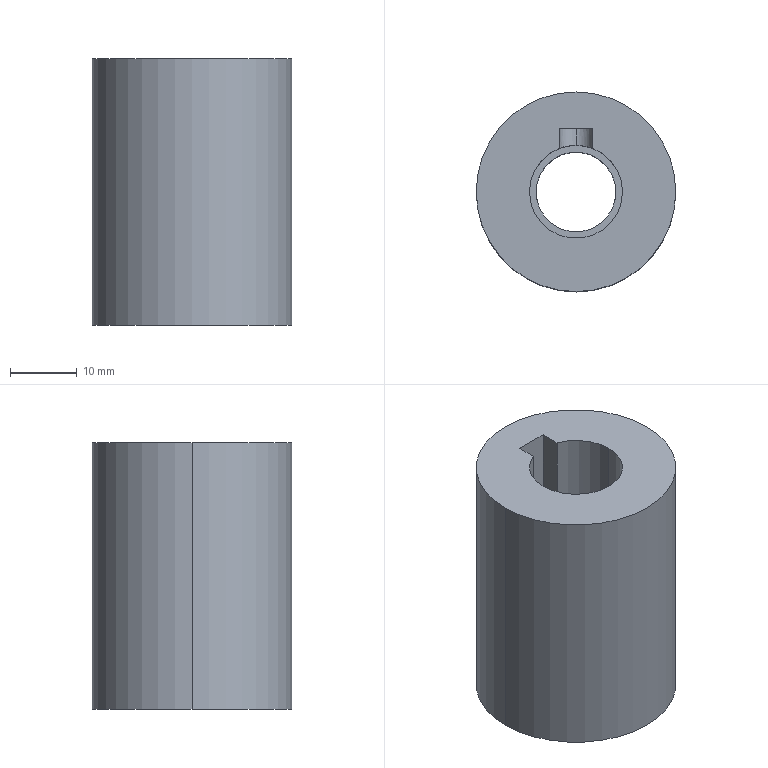Part | 1 solid | 19 faces | box 30 x 30 x 40 mm | volume 22641 mm3 | cylinder 10 | plane 9 | commonest cylinder face diameters 4 x2 5 x2 12 x2 14 x2 30 x2
STEP:
#1=CARTESIAN_POINT('',(-7.,0.,20.));
#2=VERTEX_POINT('',#1);
#3=CARTESIAN_POINT('',(7.,0.,20.));
#4=VERTEX_POINT('',#3);
#5=CARTESIAN_POINT('',(0.,0.,20.));
#6=DIRECTION('',(0.,0.,1.));
#7=DIRECTION('',(1.,0.,0.));
#8=AXIS2_PLACEMENT_3D('',#5,#6,#7);
#9=CIRCLE('',#8,7.);
#10=EDGE_CURVE('',#2,#4,#9,.T.);
#11=ORIENTED_EDGE('',*,*,#10,.T.);
#12=CARTESIAN_POINT('',(7.,0.,0.));
#13=VERTEX_POINT('',#12);
#14=CARTESIAN_POINT('',(7.,0.,20.));
#15=DIRECTION('',(0.,0.,-1.));
#16=VECTOR('',#15,1000.);
#17=LINE('',#14,#16);
#18=EDGE_CURVE('',#4,#13,#17,.T.);
#19=ORIENTED_EDGE('',*,*,#18,.T.);
#20=CARTESIAN_POINT('',(-7.,0.,0.));
#21=VERTEX_POINT('',#20);
#22=CARTESIAN_POINT('',(0.,0.,0.));
#23=DIRECTION('',(0.,0.,1.));
#24=DIRECTION('',(1.,0.,0.));
#25=AXIS2_PLACEMENT_3D('',#22,#23,#24);
#26=CIRCLE('',#25,7.);
#27=EDGE_CURVE('',#21,#13,#26,.T.);
#28=ORIENTED_EDGE('',*,*,#27,.F.);
#29=CARTESIAN_POINT('',(-7.,0.,20.));
#30=DIRECTION('',(0.,0.,-1.));
#31=VECTOR('',#30,1000.);
#32=LINE('',#29,#31);
#33=EDGE_CURVE('',#2,#21,#32,.T.);
#34=ORIENTED_EDGE('',*,*,#33,.F.);
#35=EDGE_LOOP('',(#11,#19,#28,#34));
#36=FACE_OUTER_BOUND('',#35,.T.);
#37=CARTESIAN_POINT('',(0.,0.,20.));
#38=DIRECTION('',(0.,0.,-1.));
#39=DIRECTION('',(-1.,0.,0.));
#40=AXIS2_PLACEMENT_3D('',#37,#38,#39);
#41=CYLINDRICAL_SURFACE('',#40,7.);
#42=ADVANCED_FACE('',(#36),#41,.F.);
#43=CARTESIAN_POINT('',(15.,0.,20.));
#44=VERTEX_POINT('',#43);
#45=CARTESIAN_POINT('',(-15.,0.,20.));
#46=VERTEX_POINT('',#45);
#47=CARTESIAN_POINT('',(0.,0.,20.));
#48=DIRECTION('',(0.,0.,1.));
#49=DIRECTION('',(1.,0.,0.));
#50=AXIS2_PLACEMENT_3D('',#47,#48,#49);
#51=CIRCLE('',#50,15.);
#52=EDGE_CURVE('',#44,#46,#51,.T.);
#53=ORIENTED_EDGE('',*,*,#52,.F.);
#54=CARTESIAN_POINT('',(15.,0.,-20.));
#55=VERTEX_POINT('',#54);
#56=CARTESIAN_POINT('',(15.,0.,20.));
#57=DIRECTION('',(0.,0.,-1.));
#58=VECTOR('',#57,1000.);
#59=LINE('',#56,#58);
#60=EDGE_CURVE('',#44,#55,#59,.T.);
#61=ORIENTED_EDGE('',*,*,#60,.T.);
#62=CARTESIAN_POINT('',(-15.,0.,-20.));
#63=VERTEX_POINT('',#62);
#64=CARTESIAN_POINT('',(0.,0.,-20.));
#65=DIRECTION('',(0.,0.,-1.));
#66=DIRECTION('',(-1.,0.,0.));
#67=AXIS2_PLACEMENT_3D('',#64,#65,#66);
#68=CIRCLE('',#67,15.);
#69=EDGE_CURVE('',#63,#55,#68,.T.);
#70=ORIENTED_EDGE('',*,*,#69,.F.);
#71=CARTESIAN_POINT('',(-15.,0.,20.));
#72=DIRECTION('',(0.,0.,-1.));
#73=VECTOR('',#72,1000.);
#74=LINE('',#71,#73);
#75=EDGE_CURVE('',#46,#63,#74,.T.);
#76=ORIENTED_EDGE('',*,*,#75,.F.);
#77=EDGE_LOOP('',(#53,#61,#70,#76));
#78=FACE_OUTER_BOUND('',#77,.T.);
#79=CARTESIAN_POINT('',(0.,0.,20.));
#80=DIRECTION('',(0.,0.,-1.));
#81=DIRECTION('',(-1.,0.,0.));
#82=AXIS2_PLACEMENT_3D('',#79,#80,#81);
#83=CYLINDRICAL_SURFACE('',#82,15.);
#84=ADVANCED_FACE('',(#78),#83,.T.);
#85=CARTESIAN_POINT('',(-2.,-5.657,-20.));
#86=VERTEX_POINT('',#85);
#87=CARTESIAN_POINT('',(-6.,0.,-20.));
#88=VERTEX_POINT('',#87);
#89=CARTESIAN_POINT('',(0.,0.,-20.));
#90=DIRECTION('',(0.,0.,-1.));
#91=DIRECTION('',(-1.,0.,0.));
#92=AXIS2_PLACEMENT_3D('',#89,#90,#91);
#93=CIRCLE('',#92,6.);
#94=EDGE_CURVE('',#86,#88,#93,.T.);
#95=ORIENTED_EDGE('',*,*,#94,.T.);
#96=CARTESIAN_POINT('',(-6.,0.,0.));
#97=VERTEX_POINT('',#96);
#98=CARTESIAN_POINT('',(-6.,0.,-20.));
#99=DIRECTION('',(0.,0.,1.));
#100=VECTOR('',#99,1000.);
#101=LINE('',#98,#100);
#102=EDGE_CURVE('',#88,#97,#101,.T.);
#103=ORIENTED_EDGE('',*,*,#102,.T.);
#104=CARTESIAN_POINT('',(6.,0.,0.));
#105=VERTEX_POINT('',#104);
#106=CARTESIAN_POINT('',(0.,0.,0.));
#107=DIRECTION('',(0.,0.,-1.));
#108=DIRECTION('',(-1.,0.,0.));
#109=AXIS2_PLACEMENT_3D('',#106,#107,#108);
#110=CIRCLE('',#109,6.);
#111=EDGE_CURVE('',#105,#97,#110,.T.);
#112=ORIENTED_EDGE('',*,*,#111,.F.);
#113=CARTESIAN_POINT('',(6.,0.,-20.));
#114=VERTEX_POINT('',#113);
#115=CARTESIAN_POINT('',(6.,0.,-20.));
#116=DIRECTION('',(0.,0.,1.));
#117=VECTOR('',#116,1000.);
#118=LINE('',#115,#117);
#119=EDGE_CURVE('',#114,#105,#118,.T.);
#120=ORIENTED_EDGE('',*,*,#119,.F.);
#121=CARTESIAN_POINT('',(2.,-5.657,-20.));
#122=VERTEX_POINT('',#121);
#123=CARTESIAN_POINT('',(0.,0.,-20.));
#124=DIRECTION('',(0.,0.,-1.));
#125=DIRECTION('',(-1.,0.,0.));
#126=AXIS2_PLACEMENT_3D('',#123,#124,#125);
#127=CIRCLE('',#126,6.);
#128=EDGE_CURVE('',#114,#122,#127,.T.);
#129=ORIENTED_EDGE('',*,*,#128,.T.);
#130=CARTESIAN_POINT('',(2.,-5.657,-8.));
#131=VERTEX_POINT('',#130);
#132=CARTESIAN_POINT('',(2.,-5.657,-6.));
#133=DIRECTION('',(0.,0.,-1.));
#134=VECTOR('',#133,1000.);
#135=LINE('',#132,#134);
#136=EDGE_CURVE('',#131,#122,#135,.T.);
#137=ORIENTED_EDGE('',*,*,#136,.F.);
#138=CARTESIAN_POINT('',(0.,-6.,-6.));
#139=VERTEX_POINT('',#138);
#140=CARTESIAN_POINT('',(2.,-5.657,-8.));
#141=CARTESIAN_POINT('',(2.,-5.657,-7.867));
#142=CARTESIAN_POINT('',(1.987,-5.662,-7.736));
#143=CARTESIAN_POINT('',(1.936,-5.679,-7.479));
#144=CARTESIAN_POINT('',(1.897,-5.693,-7.352));
#145=CARTESIAN_POINT('',(1.796,-5.725,-7.11));
#146=CARTESIAN_POINT('',(1.735,-5.744,-6.996));
#147=CARTESIAN_POINT('',(1.59,-5.786,-6.779));
#148=CARTESIAN_POINT('',(1.506,-5.809,-6.678));
#149=CARTESIAN_POINT('',(1.232,-5.875,-6.403));
#150=CARTESIAN_POINT('',(1.01,-5.919,-6.255));
#151=CARTESIAN_POINT('',(0.6502,-5.966,-6.104));
#152=CARTESIAN_POINT('',(0.5235,-5.979,-6.065));
#153=CARTESIAN_POINT('',(0.2644,-5.996,-6.013));
#154=CARTESIAN_POINT('',(0.1331,-6.,-6.));
#155=CARTESIAN_POINT('',(0.,-6.,-6.));
#156=B_SPLINE_CURVE_WITH_KNOTS('',3,(#140,#141,#142,#143,#144,#145,#146,#147,#148,#149,#150,#151,#152,#153,#154,#155),.UNSPECIFIED.,.F.,.F.,(4,2,2,2,2,2,2,4),(0.,0.0003934,0.0007868,0.00118,0.001574,0.00236,0.002754,0.003147),.UNSPECIFIED.);
#157=EDGE_CURVE('',#131,#139,#156,.T.);
#158=ORIENTED_EDGE('',*,*,#157,.T.);
#159=CARTESIAN_POINT('',(-2.,-5.657,-8.));
#160=VERTEX_POINT('',#159);
#161=CARTESIAN_POINT('',(0.,-6.,-6.));
#162=CARTESIAN_POINT('',(-0.1331,-6.,-6.));
#163=CARTESIAN_POINT('',(-0.2638,-5.996,-6.013));
#164=CARTESIAN_POINT('',(-0.5206,-5.979,-6.065));
#165=CARTESIAN_POINT('',(-0.6481,-5.966,-6.103));
#166=CARTESIAN_POINT('',(-0.8898,-5.935,-6.204));
#167=CARTESIAN_POINT('',(-1.004,-5.916,-6.266));
#168=CARTESIAN_POINT('',(-1.221,-5.876,-6.411));
#169=CARTESIAN_POINT('',(-1.323,-5.853,-6.494));
#170=CARTESIAN_POINT('',(-1.597,-5.787,-6.769));
#171=CARTESIAN_POINT('',(-1.746,-5.741,-6.99));
#172=CARTESIAN_POINT('',(-1.896,-5.693,-7.35));
#173=CARTESIAN_POINT('',(-1.935,-5.68,-7.477));
#174=CARTESIAN_POINT('',(-1.987,-5.662,-7.736));
#175=CARTESIAN_POINT('',(-2.,-5.657,-7.867));
#176=CARTESIAN_POINT('',(-2.,-5.657,-8.));
#177=B_SPLINE_CURVE_WITH_KNOTS('',3,(#161,#162,#163,#164,#165,#166,#167,#168,#169,#170,#171,#172,#173,#174,#175,#176),.UNSPECIFIED.,.F.,.F.,(4,2,2,2,2,2,2,4),(0.,0.0003934,0.0007868,0.00118,0.001574,0.00236,0.002754,0.003147),.UNSPECIFIED.);
#178=EDGE_CURVE('',#139,#160,#177,.T.);
#179=ORIENTED_EDGE('',*,*,#178,.T.);
#180=CARTESIAN_POINT('',(-2.,-5.657,-6.));
#181=DIRECTION('',(0.,0.,-1.));
#182=VECTOR('',#181,1000.);
#183=LINE('',#180,#182);
#184=EDGE_CURVE('',#160,#86,#183,.T.);
#185=ORIENTED_EDGE('',*,*,#184,.T.);
#186=EDGE_LOOP('',(#95,#103,#112,#120,#129,#137,#158,#179,#185));
#187=FACE_OUTER_BOUND('',#186,.T.);
#188=CARTESIAN_POINT('',(0.,0.,-20.));
#189=DIRECTION('',(0.,0.,1.));
#190=DIRECTION('',(1.,0.,0.));
#191=AXIS2_PLACEMENT_3D('',#188,#189,#190);
#192=CYLINDRICAL_SURFACE('',#191,6.);
#193=ADVANCED_FACE('',(#187),#192,.F.);
#194=ORIENTED_EDGE('',*,*,#69,.T.);
#195=CARTESIAN_POINT('',(0.,0.,-20.));
#196=DIRECTION('',(0.,0.,-1.));
#197=DIRECTION('',(-1.,0.,0.));
#198=AXIS2_PLACEMENT_3D('',#195,#196,#197);
#199=CIRCLE('',#198,15.);
#200=EDGE_CURVE('',#55,#63,#199,.T.);
#201=ORIENTED_EDGE('',*,*,#200,.T.);
#202=EDGE_LOOP('',(#194,#201));
#203=FACE_OUTER_BOUND('',#202,.T.);
#204=CARTESIAN_POINT('',(-2.,-8.,-20.));
#205=VERTEX_POINT('',#204);
#206=CARTESIAN_POINT('',(2.,-8.,-20.));
#207=VERTEX_POINT('',#206);
#208=CARTESIAN_POINT('',(0.,-8.,-20.));
#209=DIRECTION('',(1.,0.,0.));
#210=VECTOR('',#209,1000.);
#211=LINE('',#208,#210);
#212=EDGE_CURVE('',#205,#207,#211,.T.);
#213=ORIENTED_EDGE('',*,*,#212,.T.);
#214=CARTESIAN_POINT('',(2.,-8.,-20.));
#215=DIRECTION('',(0.,1.,0.));
#216=VECTOR('',#215,1000.);
#217=LINE('',#214,#216);
#218=EDGE_CURVE('',#207,#122,#217,.T.);
#219=ORIENTED_EDGE('',*,*,#218,.T.);
#220=ORIENTED_EDGE('',*,*,#128,.F.);
#221=CARTESIAN_POINT('',(0.,0.,-20.));
#222=DIRECTION('',(0.,0.,-1.));
#223=DIRECTION('',(-1.,0.,0.));
#224=AXIS2_PLACEMENT_3D('',#221,#222,#223);
#225=CIRCLE('',#224,6.);
#226=EDGE_CURVE('',#88,#114,#225,.T.);
#227=ORIENTED_EDGE('',*,*,#226,.F.);
#228=ORIENTED_EDGE('',*,*,#94,.F.);
#229=CARTESIAN_POINT('',(-2.,-8.,-20.));
#230=DIRECTION('',(0.,1.,0.));
#231=VECTOR('',#230,1000.);
#232=LINE('',#229,#231);
#233=EDGE_CURVE('',#205,#86,#232,.T.);
#234=ORIENTED_EDGE('',*,*,#233,.F.);
#235=EDGE_LOOP('',(#213,#219,#220,#227,#228,#234));
#236=FACE_BOUND('',#235,.T.);
#237=CARTESIAN_POINT('',(0.,0.,-20.));
#238=DIRECTION('',(0.,0.,-1.));
#239=DIRECTION('',(-1.,0.,0.));
#240=AXIS2_PLACEMENT_3D('',#237,#238,#239);
#241=PLANE('',#240);
#242=ADVANCED_FACE('',(#203,#236),#241,.T.);
#243=ORIENTED_EDGE('',*,*,#102,.F.);
#244=ORIENTED_EDGE('',*,*,#226,.T.);
#245=ORIENTED_EDGE('',*,*,#119,.T.);
#246=CARTESIAN_POINT('',(0.,0.,0.));
#247=DIRECTION('',(0.,0.,-1.));
#248=DIRECTION('',(-1.,0.,0.));
#249=AXIS2_PLACEMENT_3D('',#246,#247,#248);
#250=CIRCLE('',#249,6.);
#251=EDGE_CURVE('',#97,#105,#250,.T.);
#252=ORIENTED_EDGE('',*,*,#251,.F.);
#253=EDGE_LOOP('',(#243,#244,#245,#252));
#254=FACE_OUTER_BOUND('',#253,.T.);
#255=CARTESIAN_POINT('',(0.,0.,-20.));
#256=DIRECTION('',(0.,0.,1.));
#257=DIRECTION('',(1.,0.,0.));
#258=AXIS2_PLACEMENT_3D('',#255,#256,#257);
#259=CYLINDRICAL_SURFACE('',#258,6.);
#260=ADVANCED_FACE('',(#254),#259,.F.);
#261=CARTESIAN_POINT('',(2.5,6.538,20.));
#262=VERTEX_POINT('',#261);
#263=CARTESIAN_POINT('',(2.5,9.5,20.));
#264=VERTEX_POINT('',#263);
#265=CARTESIAN_POINT('',(2.5,9.5,20.));
#266=DIRECTION('',(0.,1.,0.));
#267=VECTOR('',#266,1000.);
#268=LINE('',#265,#267);
#269=EDGE_CURVE('',#262,#264,#268,.T.);
#270=ORIENTED_EDGE('',*,*,#269,.F.);
#271=CARTESIAN_POINT('',(0.,0.,20.));
#272=DIRECTION('',(0.,0.,1.));
#273=DIRECTION('',(1.,0.,0.));
#274=AXIS2_PLACEMENT_3D('',#271,#272,#273);
#275=CIRCLE('',#274,7.);
#276=EDGE_CURVE('',#4,#262,#275,.T.);
#277=ORIENTED_EDGE('',*,*,#276,.F.);
#278=ORIENTED_EDGE('',*,*,#10,.F.);
#279=CARTESIAN_POINT('',(-2.5,6.538,20.));
#280=VERTEX_POINT('',#279);
#281=CARTESIAN_POINT('',(0.,0.,20.));
#282=DIRECTION('',(0.,0.,1.));
#283=DIRECTION('',(1.,0.,0.));
#284=AXIS2_PLACEMENT_3D('',#281,#282,#283);
#285=CIRCLE('',#284,7.);
#286=EDGE_CURVE('',#280,#2,#285,.T.);
#287=ORIENTED_EDGE('',*,*,#286,.F.);
#288=CARTESIAN_POINT('',(-2.5,9.5,20.));
#289=VERTEX_POINT('',#288);
#290=CARTESIAN_POINT('',(-2.5,4.866,20.));
#291=DIRECTION('',(0.,-1.,0.));
#292=VECTOR('',#291,1000.);
#293=LINE('',#290,#292);
#294=EDGE_CURVE('',#289,#280,#293,.T.);
#295=ORIENTED_EDGE('',*,*,#294,.F.);
#296=CARTESIAN_POINT('',(0.,9.5,20.));
#297=DIRECTION('',(-1.,0.,0.));
#298=VECTOR('',#297,1000.);
#299=LINE('',#296,#298);
#300=EDGE_CURVE('',#264,#289,#299,.T.);
#301=ORIENTED_EDGE('',*,*,#300,.F.);
#302=EDGE_LOOP('',(#270,#277,#278,#287,#295,#301));
#303=FACE_BOUND('',#302,.T.);
#304=CARTESIAN_POINT('',(0.,0.,20.));
#305=DIRECTION('',(0.,0.,1.));
#306=DIRECTION('',(1.,0.,0.));
#307=AXIS2_PLACEMENT_3D('',#304,#305,#306);
#308=CIRCLE('',#307,15.);
#309=EDGE_CURVE('',#46,#44,#308,.T.);
#310=ORIENTED_EDGE('',*,*,#309,.T.);
#311=ORIENTED_EDGE('',*,*,#52,.T.);
#312=EDGE_LOOP('',(#310,#311));
#313=FACE_OUTER_BOUND('',#312,.T.);
#314=CARTESIAN_POINT('',(0.,0.,20.));
#315=DIRECTION('',(0.,0.,1.));
#316=DIRECTION('',(1.,0.,0.));
#317=AXIS2_PLACEMENT_3D('',#314,#315,#316);
#318=PLANE('',#317);
#319=ADVANCED_FACE('',(#303,#313),#318,.T.);
#320=ORIENTED_EDGE('',*,*,#60,.F.);
#321=ORIENTED_EDGE('',*,*,#309,.F.);
#322=ORIENTED_EDGE('',*,*,#75,.T.);
#323=ORIENTED_EDGE('',*,*,#200,.F.);
#324=EDGE_LOOP('',(#320,#321,#322,#323));
#325=FACE_OUTER_BOUND('',#324,.T.);
#326=CARTESIAN_POINT('',(0.,0.,20.));
#327=DIRECTION('',(0.,0.,-1.));
#328=DIRECTION('',(-1.,0.,0.));
#329=AXIS2_PLACEMENT_3D('',#326,#327,#328);
#330=CYLINDRICAL_SURFACE('',#329,15.);
#331=ADVANCED_FACE('',(#325),#330,.T.);
#332=ORIENTED_EDGE('',*,*,#18,.F.);
#333=ORIENTED_EDGE('',*,*,#276,.T.);
#334=CARTESIAN_POINT('',(2.5,6.538,8.5));
#335=VERTEX_POINT('',#334);
#336=CARTESIAN_POINT('',(2.5,6.538,20.));
#337=DIRECTION('',(0.,0.,1.));
#338=VECTOR('',#337,1000.);
#339=LINE('',#336,#338);
#340=EDGE_CURVE('',#335,#262,#339,.T.);
#341=ORIENTED_EDGE('',*,*,#340,.F.);
#342=CARTESIAN_POINT('',(0.,7.,6.));
#343=VERTEX_POINT('',#342);
#344=CARTESIAN_POINT('',(2.5,6.538,8.5));
#345=CARTESIAN_POINT('',(2.5,6.538,8.333));
#346=CARTESIAN_POINT('',(2.484,6.545,8.17));
#347=CARTESIAN_POINT('',(2.419,6.569,7.849));
#348=CARTESIAN_POINT('',(2.371,6.587,7.689));
#349=CARTESIAN_POINT('',(2.245,6.631,7.388));
#350=CARTESIAN_POINT('',(2.168,6.656,7.245));
#351=CARTESIAN_POINT('',(1.987,6.713,6.974));
#352=CARTESIAN_POINT('',(1.883,6.743,6.847));
#353=CARTESIAN_POINT('',(1.54,6.833,6.504));
#354=CARTESIAN_POINT('',(1.264,6.892,6.319));
#355=CARTESIAN_POINT('',(0.8135,6.954,6.13));
#356=CARTESIAN_POINT('',(0.6548,6.971,6.082));
#357=CARTESIAN_POINT('',(0.3308,6.994,6.016));
#358=CARTESIAN_POINT('',(0.1666,7.,6.));
#359=CARTESIAN_POINT('',(0.,7.,6.));
#360=B_SPLINE_CURVE_WITH_KNOTS('',3,(#344,#345,#346,#347,#348,#349,#350,#351,#352,#353,#354,#355,#356,#357,#358,#359),.UNSPECIFIED.,.F.,.F.,(4,2,2,2,2,2,2,4),(0.,0.0004923,0.0009846,0.001477,0.001969,0.002954,0.003446,0.003938),.UNSPECIFIED.);
#361=EDGE_CURVE('',#335,#343,#360,.T.);
#362=ORIENTED_EDGE('',*,*,#361,.T.);
#363=CARTESIAN_POINT('',(-2.5,6.538,8.5));
#364=VERTEX_POINT('',#363);
#365=CARTESIAN_POINT('',(0.,7.,6.));
#366=CARTESIAN_POINT('',(-0.1666,7.,6.));
#367=CARTESIAN_POINT('',(-0.3301,6.994,6.016));
#368=CARTESIAN_POINT('',(-0.6514,6.971,6.081));
#369=CARTESIAN_POINT('',(-0.8108,6.955,6.129));
#370=CARTESIAN_POINT('',(-1.113,6.913,6.255));
#371=CARTESIAN_POINT('',(-1.256,6.888,6.332));
#372=CARTESIAN_POINT('',(-1.527,6.833,6.514));
#373=CARTESIAN_POINT('',(-1.654,6.803,6.618));
#374=CARTESIAN_POINT('',(-1.996,6.713,6.961));
#375=CARTESIAN_POINT('',(-2.182,6.653,7.237));
#376=CARTESIAN_POINT('',(-2.37,6.587,7.687));
#377=CARTESIAN_POINT('',(-2.418,6.569,7.845));
#378=CARTESIAN_POINT('',(-2.484,6.545,8.169));
#379=CARTESIAN_POINT('',(-2.5,6.538,8.333));
#380=CARTESIAN_POINT('',(-2.5,6.538,8.5));
#381=B_SPLINE_CURVE_WITH_KNOTS('',3,(#365,#366,#367,#368,#369,#370,#371,#372,#373,#374,#375,#376,#377,#378,#379,#380),.UNSPECIFIED.,.F.,.F.,(4,2,2,2,2,2,2,4),(0.,0.0004923,0.0009846,0.001477,0.001969,0.002954,0.003446,0.003938),.UNSPECIFIED.);
#382=EDGE_CURVE('',#343,#364,#381,.T.);
#383=ORIENTED_EDGE('',*,*,#382,.T.);
#384=CARTESIAN_POINT('',(-2.5,6.538,20.));
#385=DIRECTION('',(0.,0.,-1.));
#386=VECTOR('',#385,1000.);
#387=LINE('',#384,#386);
#388=EDGE_CURVE('',#280,#364,#387,.T.);
#389=ORIENTED_EDGE('',*,*,#388,.F.);
#390=ORIENTED_EDGE('',*,*,#286,.T.);
#391=ORIENTED_EDGE('',*,*,#33,.T.);
#392=CARTESIAN_POINT('',(0.,0.,0.));
#393=DIRECTION('',(0.,0.,1.));
#394=DIRECTION('',(1.,0.,0.));
#395=AXIS2_PLACEMENT_3D('',#392,#393,#394);
#396=CIRCLE('',#395,7.);
#397=EDGE_CURVE('',#13,#21,#396,.T.);
#398=ORIENTED_EDGE('',*,*,#397,.F.);
#399=EDGE_LOOP('',(#332,#333,#341,#362,#383,#389,#390,#391,#398));
#400=FACE_OUTER_BOUND('',#399,.T.);
#401=CARTESIAN_POINT('',(0.,0.,20.));
#402=DIRECTION('',(0.,0.,-1.));
#403=DIRECTION('',(-1.,0.,0.));
#404=AXIS2_PLACEMENT_3D('',#401,#402,#403);
#405=CYLINDRICAL_SURFACE('',#404,7.);
#406=ADVANCED_FACE('',(#400),#405,.F.);
#407=ORIENTED_EDGE('',*,*,#27,.T.);
#408=ORIENTED_EDGE('',*,*,#397,.T.);
#409=EDGE_LOOP('',(#407,#408));
#410=FACE_OUTER_BOUND('',#409,.T.);
#411=ORIENTED_EDGE('',*,*,#111,.T.);
#412=ORIENTED_EDGE('',*,*,#251,.T.);
#413=EDGE_LOOP('',(#411,#412));
#414=FACE_BOUND('',#413,.T.);
#415=CARTESIAN_POINT('',(0.,0.,0.));
#416=DIRECTION('',(0.,0.,-1.));
#417=DIRECTION('',(-1.,0.,0.));
#418=AXIS2_PLACEMENT_3D('',#415,#416,#417);
#419=PLANE('',#418);
#420=ADVANCED_FACE('',(#410,#414),#419,.F.);
#421=CARTESIAN_POINT('',(-2.5,9.5,8.5));
#422=VERTEX_POINT('',#421);
#423=CARTESIAN_POINT('',(0.,9.5,6.));
#424=VERTEX_POINT('',#423);
#425=CARTESIAN_POINT('',(0.,9.5,8.5));
#426=DIRECTION('',(0.,-1.,0.));
#427=DIRECTION('',(0.,0.,1.));
#428=AXIS2_PLACEMENT_3D('',#425,#426,#427);
#429=CIRCLE('',#428,2.5);
#430=EDGE_CURVE('',#422,#424,#429,.T.);
#431=ORIENTED_EDGE('',*,*,#430,.T.);
#432=CARTESIAN_POINT('',(2.5,9.5,8.5));
#433=VERTEX_POINT('',#432);
#434=CARTESIAN_POINT('',(0.,9.5,8.5));
#435=DIRECTION('',(0.,-1.,0.));
#436=DIRECTION('',(0.,0.,1.));
#437=AXIS2_PLACEMENT_3D('',#434,#435,#436);
#438=CIRCLE('',#437,2.5);
#439=EDGE_CURVE('',#424,#433,#438,.T.);
#440=ORIENTED_EDGE('',*,*,#439,.T.);
#441=CARTESIAN_POINT('',(2.5,9.5,6.));
#442=DIRECTION('',(0.,0.,1.));
#443=VECTOR('',#442,1000.);
#444=LINE('',#441,#443);
#445=EDGE_CURVE('',#433,#264,#444,.T.);
#446=ORIENTED_EDGE('',*,*,#445,.T.);
#447=ORIENTED_EDGE('',*,*,#300,.T.);
#448=CARTESIAN_POINT('',(-2.5,9.5,6.));
#449=DIRECTION('',(0.,0.,1.));
#450=VECTOR('',#449,1000.);
#451=LINE('',#448,#450);
#452=EDGE_CURVE('',#422,#289,#451,.T.);
#453=ORIENTED_EDGE('',*,*,#452,.F.);
#454=EDGE_LOOP('',(#431,#440,#446,#447,#453));
#455=FACE_OUTER_BOUND('',#454,.T.);
#456=CARTESIAN_POINT('',(0.,9.5,6.));
#457=DIRECTION('',(0.,1.,0.));
#458=DIRECTION('',(0.,0.,1.));
#459=AXIS2_PLACEMENT_3D('',#456,#457,#458);
#460=PLANE('',#459);
#461=ADVANCED_FACE('',(#455),#460,.F.);
#462=ORIENTED_EDGE('',*,*,#445,.F.);
#463=CARTESIAN_POINT('',(2.5,6.538,8.5));
#464=DIRECTION('',(0.,-1.,0.));
#465=VECTOR('',#464,1000.);
#466=LINE('',#463,#465);
#467=EDGE_CURVE('',#433,#335,#466,.T.);
#468=ORIENTED_EDGE('',*,*,#467,.T.);
#469=ORIENTED_EDGE('',*,*,#340,.T.);
#470=ORIENTED_EDGE('',*,*,#269,.T.);
#471=EDGE_LOOP('',(#462,#468,#469,#470));
#472=FACE_OUTER_BOUND('',#471,.T.);
#473=CARTESIAN_POINT('',(2.5,9.5,6.));
#474=DIRECTION('',(1.,0.,0.));
#475=DIRECTION('',(0.,1.,0.));
#476=AXIS2_PLACEMENT_3D('',#473,#474,#475);
#477=PLANE('',#476);
#478=ADVANCED_FACE('',(#472),#477,.F.);
#479=ORIENTED_EDGE('',*,*,#388,.T.);
#480=CARTESIAN_POINT('',(-2.5,9.5,8.5));
#481=DIRECTION('',(0.,1.,0.));
#482=VECTOR('',#481,1000.);
#483=LINE('',#480,#482);
#484=EDGE_CURVE('',#364,#422,#483,.T.);
#485=ORIENTED_EDGE('',*,*,#484,.T.);
#486=ORIENTED_EDGE('',*,*,#452,.T.);
#487=ORIENTED_EDGE('',*,*,#294,.T.);
#488=EDGE_LOOP('',(#479,#485,#486,#487));
#489=FACE_OUTER_BOUND('',#488,.T.);
#490=CARTESIAN_POINT('',(-2.5,4.866,6.));
#491=DIRECTION('',(-1.,0.,0.));
#492=DIRECTION('',(0.,0.,1.));
#493=AXIS2_PLACEMENT_3D('',#490,#491,#492);
#494=PLANE('',#493);
#495=ADVANCED_FACE('',(#489),#494,.F.);
#496=ORIENTED_EDGE('',*,*,#484,.F.);
#497=ORIENTED_EDGE('',*,*,#382,.F.);
#498=CARTESIAN_POINT('',(0.,6.538,6.));
#499=DIRECTION('',(0.,-1.,0.));
#500=VECTOR('',#499,1000.);
#501=LINE('',#498,#500);
#502=EDGE_CURVE('',#424,#343,#501,.T.);
#503=ORIENTED_EDGE('',*,*,#502,.F.);
#504=ORIENTED_EDGE('',*,*,#430,.F.);
#505=EDGE_LOOP('',(#496,#497,#503,#504));
#506=FACE_OUTER_BOUND('',#505,.T.);
#507=CARTESIAN_POINT('',(0.,0.,8.5));
#508=DIRECTION('',(0.,1.,0.));
#509=DIRECTION('',(0.,0.,1.));
#510=AXIS2_PLACEMENT_3D('',#507,#508,#509);
#511=CYLINDRICAL_SURFACE('',#510,2.5);
#512=ADVANCED_FACE('',(#506),#511,.F.);
#513=ORIENTED_EDGE('',*,*,#361,.F.);
#514=ORIENTED_EDGE('',*,*,#467,.F.);
#515=ORIENTED_EDGE('',*,*,#439,.F.);
#516=ORIENTED_EDGE('',*,*,#502,.T.);
#517=EDGE_LOOP('',(#513,#514,#515,#516));
#518=FACE_OUTER_BOUND('',#517,.T.);
#519=CARTESIAN_POINT('',(0.,0.,8.5));
#520=DIRECTION('',(0.,-1.,0.));
#521=DIRECTION('',(1.,0.,0.));
#522=AXIS2_PLACEMENT_3D('',#519,#520,#521);
#523=CYLINDRICAL_SURFACE('',#522,2.5);
#524=ADVANCED_FACE('',(#518),#523,.F.);
#525=CARTESIAN_POINT('',(2.,-8.,-8.));
#526=VERTEX_POINT('',#525);
#527=CARTESIAN_POINT('',(2.,-8.,-6.));
#528=DIRECTION('',(0.,0.,-1.));
#529=VECTOR('',#528,1000.);
#530=LINE('',#527,#529);
#531=EDGE_CURVE('',#526,#207,#530,.T.);
#532=ORIENTED_EDGE('',*,*,#531,.F.);
#533=CARTESIAN_POINT('',(2.,-8.,-8.));
#534=DIRECTION('',(0.,1.,0.));
#535=VECTOR('',#534,1000.);
#536=LINE('',#533,#535);
#537=EDGE_CURVE('',#526,#131,#536,.T.);
#538=ORIENTED_EDGE('',*,*,#537,.T.);
#539=ORIENTED_EDGE('',*,*,#136,.T.);
#540=ORIENTED_EDGE('',*,*,#218,.F.);
#541=EDGE_LOOP('',(#532,#538,#539,#540));
#542=FACE_OUTER_BOUND('',#541,.T.);
#543=CARTESIAN_POINT('',(2.,-8.,-6.));
#544=DIRECTION('',(-1.,0.,0.));
#545=DIRECTION('',(0.,0.,1.));
#546=AXIS2_PLACEMENT_3D('',#543,#544,#545);
#547=PLANE('',#546);
#548=ADVANCED_FACE('',(#542),#547,.T.);
#549=ORIENTED_EDGE('',*,*,#184,.F.);
#550=CARTESIAN_POINT('',(-2.,-8.,-8.));
#551=VERTEX_POINT('',#550);
#552=CARTESIAN_POINT('',(-2.,-8.,-8.));
#553=DIRECTION('',(0.,-1.,0.));
#554=VECTOR('',#553,1000.);
#555=LINE('',#552,#554);
#556=EDGE_CURVE('',#160,#551,#555,.T.);
#557=ORIENTED_EDGE('',*,*,#556,.T.);
#558=CARTESIAN_POINT('',(-2.,-8.,-6.));
#559=DIRECTION('',(0.,0.,-1.));
#560=VECTOR('',#559,1000.);
#561=LINE('',#558,#560);
#562=EDGE_CURVE('',#551,#205,#561,.T.);
#563=ORIENTED_EDGE('',*,*,#562,.T.);
#564=ORIENTED_EDGE('',*,*,#233,.T.);
#565=EDGE_LOOP('',(#549,#557,#563,#564));
#566=FACE_OUTER_BOUND('',#565,.T.);
#567=CARTESIAN_POINT('',(-2.,-8.,-6.));
#568=DIRECTION('',(-1.,0.,0.));
#569=DIRECTION('',(0.,-1.,0.));
#570=AXIS2_PLACEMENT_3D('',#567,#568,#569);
#571=PLANE('',#570);
#572=ADVANCED_FACE('',(#566),#571,.F.);
#573=ORIENTED_EDGE('',*,*,#562,.F.);
#574=CARTESIAN_POINT('',(0.,-8.,-6.));
#575=VERTEX_POINT('',#574);
#576=CARTESIAN_POINT('',(0.,-8.,-8.));
#577=DIRECTION('',(0.,1.,0.));
#578=DIRECTION('',(0.,0.,1.));
#579=AXIS2_PLACEMENT_3D('',#576,#577,#578);
#580=CIRCLE('',#579,2.);
#581=EDGE_CURVE('',#551,#575,#580,.T.);
#582=ORIENTED_EDGE('',*,*,#581,.T.);
#583=CARTESIAN_POINT('',(0.,-8.,-8.));
#584=DIRECTION('',(0.,1.,0.));
#585=DIRECTION('',(0.,0.,1.));
#586=AXIS2_PLACEMENT_3D('',#583,#584,#585);
#587=CIRCLE('',#586,2.);
#588=EDGE_CURVE('',#575,#526,#587,.T.);
#589=ORIENTED_EDGE('',*,*,#588,.T.);
#590=ORIENTED_EDGE('',*,*,#531,.T.);
#591=ORIENTED_EDGE('',*,*,#212,.F.);
#592=EDGE_LOOP('',(#573,#582,#589,#590,#591));
#593=FACE_OUTER_BOUND('',#592,.T.);
#594=CARTESIAN_POINT('',(0.,-8.,-6.));
#595=DIRECTION('',(0.,1.,0.));
#596=DIRECTION('',(0.,0.,1.));
#597=AXIS2_PLACEMENT_3D('',#594,#595,#596);
#598=PLANE('',#597);
#599=ADVANCED_FACE('',(#593),#598,.T.);
#600=ORIENTED_EDGE('',*,*,#537,.F.);
#601=ORIENTED_EDGE('',*,*,#588,.F.);
#602=CARTESIAN_POINT('',(0.,0.,-6.));
#603=DIRECTION('',(0.,-1.,0.));
#604=VECTOR('',#603,1000.);
#605=LINE('',#602,#604);
#606=EDGE_CURVE('',#139,#575,#605,.T.);
#607=ORIENTED_EDGE('',*,*,#606,.F.);
#608=ORIENTED_EDGE('',*,*,#157,.F.);
#609=EDGE_LOOP('',(#600,#601,#607,#608));
#610=FACE_OUTER_BOUND('',#609,.T.);
#611=CARTESIAN_POINT('',(0.,-8.,-8.));
#612=DIRECTION('',(0.,1.,0.));
#613=DIRECTION('',(0.,0.,1.));
#614=AXIS2_PLACEMENT_3D('',#611,#612,#613);
#615=CYLINDRICAL_SURFACE('',#614,2.);
#616=ADVANCED_FACE('',(#610),#615,.F.);
#617=ORIENTED_EDGE('',*,*,#581,.F.);
#618=ORIENTED_EDGE('',*,*,#556,.F.);
#619=ORIENTED_EDGE('',*,*,#178,.F.);
#620=ORIENTED_EDGE('',*,*,#606,.T.);
#621=EDGE_LOOP('',(#617,#618,#619,#620));
#622=FACE_OUTER_BOUND('',#621,.T.);
#623=CARTESIAN_POINT('',(0.,0.,-8.));
#624=DIRECTION('',(0.,-1.,0.));
#625=DIRECTION('',(1.,0.,0.));
#626=AXIS2_PLACEMENT_3D('',#623,#624,#625);
#627=CYLINDRICAL_SURFACE('',#626,2.);
#628=ADVANCED_FACE('',(#622),#627,.F.);
#629=CLOSED_SHELL('',(#42,#84,#193,#242,#260,#319,#331,#406,#420,#461,#478,#495,#512,#524,#548,#572,#599,#616,#628));
#630=MANIFOLD_SOLID_BREP('',#629);
#631=CARTESIAN_POINT('',(0.,0.,0.));
#632=DIRECTION('',(0.,0.,1.));
#633=DIRECTION('',(1.,0.,0.));
#634=AXIS2_PLACEMENT_3D('',#631,#632,#633);
#635=(LENGTH_UNIT()NAMED_UNIT(*)SI_UNIT(.MILLI.,.METRE.));
#636=UNCERTAINTY_MEASURE_WITH_UNIT(LENGTH_MEASURE(0.00001),#635,'','');
#637=(NAMED_UNIT(*)PLANE_ANGLE_UNIT()SI_UNIT($,.RADIAN.));
#638=(NAMED_UNIT(*)SI_UNIT($,.STERADIAN.)SOLID_ANGLE_UNIT());
#639=(GEOMETRIC_REPRESENTATION_CONTEXT(3)GLOBAL_UNCERTAINTY_ASSIGNED_CONTEXT((#636))GLOBAL_UNIT_ASSIGNED_CONTEXT((#635,#637,#638))REPRESENTATION_CONTEXT('',''));
#640=ADVANCED_BREP_SHAPE_REPRESENTATION('',(#630,#634),#639);